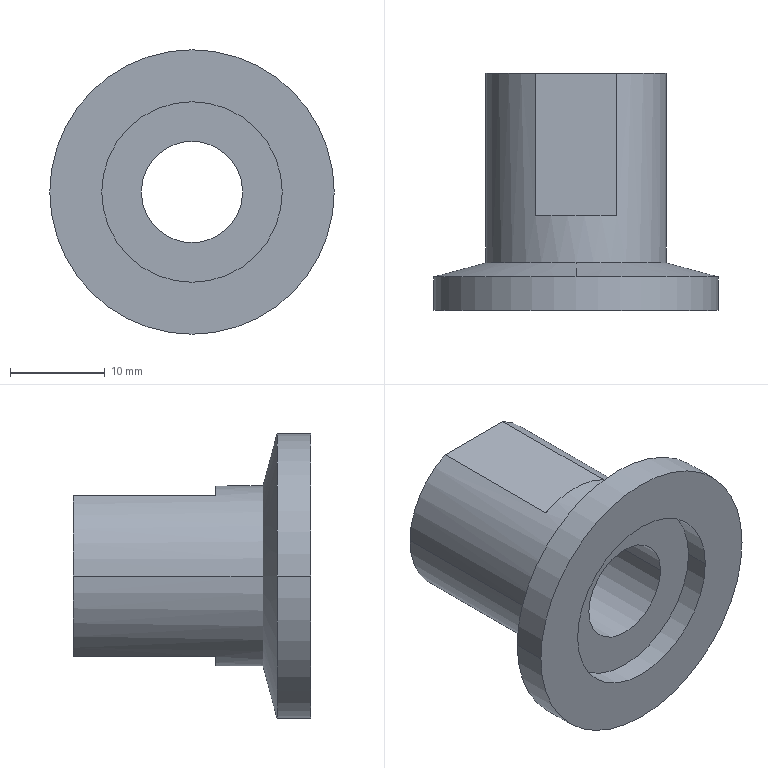Part | SolidWorks | features BaseBody 1 | 1 solid | 20 faces | box 30 x 25 x 30 mm | volume 5740 mm3 | cylinder 8 | plane 8 | cone 4 | commonest cylinder face diameters 19.05 x4 10.7 x2 30 x2
STEP:
#1=CARTESIAN_POINT('',(0.,5.,9.525));
#2=VERTEX_POINT('',#1);
#3=CARTESIAN_POINT('',(9.525,5.,0.));
#4=VERTEX_POINT('',#3);
#5=CARTESIAN_POINT('',(0.,5.,0.));
#6=DIRECTION('',(0.,1.,0.));
#7=DIRECTION('',(-1.,0.,0.));
#8=AXIS2_PLACEMENT_3D('',#5,#6,#7);
#9=CIRCLE('',#8,9.525);
#10=EDGE_CURVE('',#2,#4,#9,.T.);
#11=ORIENTED_EDGE('',*,*,#10,.T.);
#12=CARTESIAN_POINT('',(9.525,25.,0.));
#13=VERTEX_POINT('',#12);
#14=CARTESIAN_POINT('',(9.525,88.82,0.));
#15=DIRECTION('',(0.,1.,0.));
#16=VECTOR('',#15,1000.);
#17=LINE('',#14,#16);
#18=EDGE_CURVE('',#4,#13,#17,.T.);
#19=ORIENTED_EDGE('',*,*,#18,.T.);
#20=CARTESIAN_POINT('',(4.298,25.,8.5));
#21=VERTEX_POINT('',#20);
#22=CARTESIAN_POINT('',(0.,25.,0.));
#23=DIRECTION('',(0.,1.,0.));
#24=DIRECTION('',(-1.,0.,0.));
#25=AXIS2_PLACEMENT_3D('',#22,#23,#24);
#26=CIRCLE('',#25,9.525);
#27=EDGE_CURVE('',#21,#13,#26,.T.);
#28=ORIENTED_EDGE('',*,*,#27,.F.);
#29=CARTESIAN_POINT('',(4.298,10.,8.5));
#30=VERTEX_POINT('',#29);
#31=CARTESIAN_POINT('',(4.298,10.,8.5));
#32=DIRECTION('',(0.,-1.,0.));
#33=VECTOR('',#32,1000.);
#34=LINE('',#31,#33);
#35=EDGE_CURVE('',#21,#30,#34,.T.);
#36=ORIENTED_EDGE('',*,*,#35,.T.);
#37=CARTESIAN_POINT('',(-4.298,10.,8.5));
#38=VERTEX_POINT('',#37);
#39=CARTESIAN_POINT('',(0.,10.,0.));
#40=DIRECTION('',(0.,-1.,0.));
#41=DIRECTION('',(-1.,0.,0.));
#42=AXIS2_PLACEMENT_3D('',#39,#40,#41);
#43=CIRCLE('',#42,9.525);
#44=EDGE_CURVE('',#30,#38,#43,.T.);
#45=ORIENTED_EDGE('',*,*,#44,.T.);
#46=CARTESIAN_POINT('',(-4.298,25.,8.5));
#47=VERTEX_POINT('',#46);
#48=CARTESIAN_POINT('',(-4.298,88.82,8.5));
#49=DIRECTION('',(0.,1.,0.));
#50=VECTOR('',#49,1000.);
#51=LINE('',#48,#50);
#52=EDGE_CURVE('',#38,#47,#51,.T.);
#53=ORIENTED_EDGE('',*,*,#52,.T.);
#54=CARTESIAN_POINT('',(-9.525,25.,0.));
#55=VERTEX_POINT('',#54);
#56=CARTESIAN_POINT('',(0.,25.,0.));
#57=DIRECTION('',(0.,-1.,0.));
#58=DIRECTION('',(-1.,0.,0.));
#59=AXIS2_PLACEMENT_3D('',#56,#57,#58);
#60=CIRCLE('',#59,9.525);
#61=EDGE_CURVE('',#47,#55,#60,.T.);
#62=ORIENTED_EDGE('',*,*,#61,.T.);
#63=CARTESIAN_POINT('',(-9.525,5.,0.));
#64=VERTEX_POINT('',#63);
#65=CARTESIAN_POINT('',(-9.525,88.82,0.));
#66=DIRECTION('',(0.,1.,0.));
#67=VECTOR('',#66,1000.);
#68=LINE('',#65,#67);
#69=EDGE_CURVE('',#64,#55,#68,.T.);
#70=ORIENTED_EDGE('',*,*,#69,.F.);
#71=CARTESIAN_POINT('',(0.,5.,0.));
#72=DIRECTION('',(0.,1.,0.));
#73=DIRECTION('',(-1.,0.,0.));
#74=AXIS2_PLACEMENT_3D('',#71,#72,#73);
#75=CIRCLE('',#74,9.525);
#76=EDGE_CURVE('',#64,#2,#75,.T.);
#77=ORIENTED_EDGE('',*,*,#76,.T.);
#78=EDGE_LOOP('',(#11,#19,#28,#36,#45,#53,#62,#70,#77));
#79=FACE_OUTER_BOUND('',#78,.T.);
#80=CARTESIAN_POINT('',(0.,88.82,0.));
#81=DIRECTION('',(0.,1.,0.));
#82=DIRECTION('',(-1.,0.,0.));
#83=AXIS2_PLACEMENT_3D('',#80,#81,#82);
#84=CYLINDRICAL_SURFACE('',#83,9.525);
#85=ADVANCED_FACE('',(#79),#84,.T.);
#86=ORIENTED_EDGE('',*,*,#10,.F.);
#87=CARTESIAN_POINT('',(0.,3.533,15.));
#88=VERTEX_POINT('',#87);
#89=CARTESIAN_POINT('',(0.,3.533,15.));
#90=DIRECTION('',(0.,-0.2588,0.9659));
#91=VECTOR('',#90,1000.);
#92=LINE('',#89,#91);
#93=EDGE_CURVE('',#2,#88,#92,.T.);
#94=ORIENTED_EDGE('',*,*,#93,.T.);
#95=CARTESIAN_POINT('',(15.,3.533,0.));
#96=VERTEX_POINT('',#95);
#97=CARTESIAN_POINT('',(0.,3.533,0.));
#98=DIRECTION('',(0.,1.,0.));
#99=DIRECTION('',(0.,0.,-1.));
#100=AXIS2_PLACEMENT_3D('',#97,#98,#99);
#101=CIRCLE('',#100,15.);
#102=EDGE_CURVE('',#88,#96,#101,.T.);
#103=ORIENTED_EDGE('',*,*,#102,.T.);
#104=CARTESIAN_POINT('',(0.,3.533,-15.));
#105=VERTEX_POINT('',#104);
#106=CARTESIAN_POINT('',(0.,3.533,0.));
#107=DIRECTION('',(0.,1.,0.));
#108=DIRECTION('',(0.,0.,-1.));
#109=AXIS2_PLACEMENT_3D('',#106,#107,#108);
#110=CIRCLE('',#109,15.);
#111=EDGE_CURVE('',#96,#105,#110,.T.);
#112=ORIENTED_EDGE('',*,*,#111,.T.);
#113=CARTESIAN_POINT('',(0.,5.,-9.525));
#114=VERTEX_POINT('',#113);
#115=CARTESIAN_POINT('',(0.,3.533,-15.));
#116=DIRECTION('',(0.,-0.2588,-0.9659));
#117=VECTOR('',#116,1000.);
#118=LINE('',#115,#117);
#119=EDGE_CURVE('',#114,#105,#118,.T.);
#120=ORIENTED_EDGE('',*,*,#119,.F.);
#121=CARTESIAN_POINT('',(0.,5.,0.));
#122=DIRECTION('',(0.,1.,0.));
#123=DIRECTION('',(-1.,0.,0.));
#124=AXIS2_PLACEMENT_3D('',#121,#122,#123);
#125=CIRCLE('',#124,9.525);
#126=EDGE_CURVE('',#4,#114,#125,.T.);
#127=ORIENTED_EDGE('',*,*,#126,.F.);
#128=EDGE_LOOP('',(#86,#94,#103,#112,#120,#127));
#129=FACE_OUTER_BOUND('',#128,.T.);
#130=CARTESIAN_POINT('',(0.,3.533,0.));
#131=DIRECTION('',(0.,-1.,0.));
#132=DIRECTION('',(0.,0.,-1.));
#133=AXIS2_PLACEMENT_3D('',#130,#131,#132);
#134=CONICAL_SURFACE('',#133,15.,1.309);
#135=ADVANCED_FACE('',(#129),#134,.T.);
#136=CARTESIAN_POINT('',(5.811,14.,0.));
#137=VERTEX_POINT('',#136);
#138=CARTESIAN_POINT('',(-5.811,14.,0.));
#139=VERTEX_POINT('',#138);
#140=CARTESIAN_POINT('',(0.,14.,0.));
#141=DIRECTION('',(0.,1.,0.));
#142=DIRECTION('',(-1.,0.,0.));
#143=AXIS2_PLACEMENT_3D('',#140,#141,#142);
#144=CIRCLE('',#143,5.811);
#145=EDGE_CURVE('',#137,#139,#144,.T.);
#146=ORIENTED_EDGE('',*,*,#145,.F.);
#147=CARTESIAN_POINT('',(6.154,25.,0.));
#148=VERTEX_POINT('',#147);
#149=CARTESIAN_POINT('',(6.154,25.,0.));
#150=DIRECTION('',(0.0312,0.9995,0.));
#151=VECTOR('',#150,1000.);
#152=LINE('',#149,#151);
#153=EDGE_CURVE('',#137,#148,#152,.T.);
#154=ORIENTED_EDGE('',*,*,#153,.T.);
#155=CARTESIAN_POINT('',(-6.154,25.,0.));
#156=VERTEX_POINT('',#155);
#157=CARTESIAN_POINT('',(0.,25.,0.));
#158=DIRECTION('',(0.,-1.,0.));
#159=DIRECTION('',(-1.,0.,0.));
#160=AXIS2_PLACEMENT_3D('',#157,#158,#159);
#161=CIRCLE('',#160,6.154);
#162=EDGE_CURVE('',#156,#148,#161,.T.);
#163=ORIENTED_EDGE('',*,*,#162,.F.);
#164=CARTESIAN_POINT('',(-6.154,25.,0.));
#165=DIRECTION('',(-0.0312,0.9995,0.));
#166=VECTOR('',#165,1000.);
#167=LINE('',#164,#166);
#168=EDGE_CURVE('',#139,#156,#167,.T.);
#169=ORIENTED_EDGE('',*,*,#168,.F.);
#170=EDGE_LOOP('',(#146,#154,#163,#169));
#171=FACE_OUTER_BOUND('',#170,.T.);
#172=CARTESIAN_POINT('',(0.,25.,0.));
#173=DIRECTION('',(0.,1.,0.));
#174=DIRECTION('',(-1.,0.,0.));
#175=AXIS2_PLACEMENT_3D('',#172,#173,#174);
#176=CONICAL_SURFACE('',#175,6.154,0.03121);
#177=ADVANCED_FACE('',(#171),#176,.F.);
#178=CARTESIAN_POINT('',(-15.,0.,0.));
#179=VERTEX_POINT('',#178);
#180=CARTESIAN_POINT('',(15.,0.,0.));
#181=VERTEX_POINT('',#180);
#182=CARTESIAN_POINT('',(0.,0.,0.));
#183=DIRECTION('',(0.,1.,0.));
#184=DIRECTION('',(-1.,0.,0.));
#185=AXIS2_PLACEMENT_3D('',#182,#183,#184);
#186=CIRCLE('',#185,15.);
#187=EDGE_CURVE('',#179,#181,#186,.T.);
#188=ORIENTED_EDGE('',*,*,#187,.T.);
#189=CARTESIAN_POINT('',(15.,88.82,0.));
#190=DIRECTION('',(0.,1.,0.));
#191=VECTOR('',#190,1000.);
#192=LINE('',#189,#191);
#193=EDGE_CURVE('',#181,#96,#192,.T.);
#194=ORIENTED_EDGE('',*,*,#193,.T.);
#195=ORIENTED_EDGE('',*,*,#102,.F.);
#196=CARTESIAN_POINT('',(-15.,3.533,0.));
#197=VERTEX_POINT('',#196);
#198=CARTESIAN_POINT('',(0.,3.533,0.));
#199=DIRECTION('',(0.,1.,0.));
#200=DIRECTION('',(0.,0.,-1.));
#201=AXIS2_PLACEMENT_3D('',#198,#199,#200);
#202=CIRCLE('',#201,15.);
#203=EDGE_CURVE('',#197,#88,#202,.T.);
#204=ORIENTED_EDGE('',*,*,#203,.F.);
#205=CARTESIAN_POINT('',(-15.,88.82,0.));
#206=DIRECTION('',(0.,1.,0.));
#207=VECTOR('',#206,1000.);
#208=LINE('',#205,#207);
#209=EDGE_CURVE('',#179,#197,#208,.T.);
#210=ORIENTED_EDGE('',*,*,#209,.F.);
#211=EDGE_LOOP('',(#188,#194,#195,#204,#210));
#212=FACE_OUTER_BOUND('',#211,.T.);
#213=CARTESIAN_POINT('',(0.,88.82,0.));
#214=DIRECTION('',(0.,1.,0.));
#215=DIRECTION('',(-1.,0.,0.));
#216=AXIS2_PLACEMENT_3D('',#213,#214,#215);
#217=CYLINDRICAL_SURFACE('',#216,15.);
#218=ADVANCED_FACE('',(#212),#217,.T.);
#219=CARTESIAN_POINT('',(5.35,2.5,0.));
#220=VERTEX_POINT('',#219);
#221=CARTESIAN_POINT('',(-5.35,2.5,0.));
#222=VERTEX_POINT('',#221);
#223=CARTESIAN_POINT('',(0.,2.5,0.));
#224=DIRECTION('',(0.,1.,0.));
#225=DIRECTION('',(-1.,0.,0.));
#226=AXIS2_PLACEMENT_3D('',#223,#224,#225);
#227=CIRCLE('',#226,5.35);
#228=EDGE_CURVE('',#220,#222,#227,.T.);
#229=ORIENTED_EDGE('',*,*,#228,.F.);
#230=CARTESIAN_POINT('',(5.35,14.,0.));
#231=VERTEX_POINT('',#230);
#232=CARTESIAN_POINT('',(5.35,25.,0.));
#233=DIRECTION('',(0.,1.,0.));
#234=VECTOR('',#233,1000.);
#235=LINE('',#232,#234);
#236=EDGE_CURVE('',#220,#231,#235,.T.);
#237=ORIENTED_EDGE('',*,*,#236,.T.);
#238=CARTESIAN_POINT('',(-5.35,14.,0.));
#239=VERTEX_POINT('',#238);
#240=CARTESIAN_POINT('',(0.,14.,0.));
#241=DIRECTION('',(0.,1.,0.));
#242=DIRECTION('',(-1.,0.,0.));
#243=AXIS2_PLACEMENT_3D('',#240,#241,#242);
#244=CIRCLE('',#243,5.35);
#245=EDGE_CURVE('',#231,#239,#244,.T.);
#246=ORIENTED_EDGE('',*,*,#245,.T.);
#247=CARTESIAN_POINT('',(-5.35,25.,0.));
#248=DIRECTION('',(0.,1.,0.));
#249=VECTOR('',#248,1000.);
#250=LINE('',#247,#249);
#251=EDGE_CURVE('',#222,#239,#250,.T.);
#252=ORIENTED_EDGE('',*,*,#251,.F.);
#253=EDGE_LOOP('',(#229,#237,#246,#252));
#254=FACE_OUTER_BOUND('',#253,.T.);
#255=CARTESIAN_POINT('',(0.,25.,0.));
#256=DIRECTION('',(0.,1.,0.));
#257=DIRECTION('',(-1.,0.,0.));
#258=AXIS2_PLACEMENT_3D('',#255,#256,#257);
#259=CYLINDRICAL_SURFACE('',#258,5.35);
#260=ADVANCED_FACE('',(#254),#259,.F.);
#261=CARTESIAN_POINT('',(9.525,0.,0.));
#262=VERTEX_POINT('',#261);
#263=CARTESIAN_POINT('',(-9.525,0.,0.));
#264=VERTEX_POINT('',#263);
#265=CARTESIAN_POINT('',(0.,0.,0.));
#266=DIRECTION('',(0.,1.,0.));
#267=DIRECTION('',(-1.,0.,0.));
#268=AXIS2_PLACEMENT_3D('',#265,#266,#267);
#269=CIRCLE('',#268,9.525);
#270=EDGE_CURVE('',#262,#264,#269,.T.);
#271=ORIENTED_EDGE('',*,*,#270,.F.);
#272=CARTESIAN_POINT('',(9.525,2.5,0.));
#273=VERTEX_POINT('',#272);
#274=CARTESIAN_POINT('',(9.525,88.82,0.));
#275=DIRECTION('',(0.,1.,0.));
#276=VECTOR('',#275,1000.);
#277=LINE('',#274,#276);
#278=EDGE_CURVE('',#262,#273,#277,.T.);
#279=ORIENTED_EDGE('',*,*,#278,.T.);
#280=CARTESIAN_POINT('',(-9.525,2.5,0.));
#281=VERTEX_POINT('',#280);
#282=CARTESIAN_POINT('',(0.,2.5,0.));
#283=DIRECTION('',(0.,-1.,0.));
#284=DIRECTION('',(-1.,0.,0.));
#285=AXIS2_PLACEMENT_3D('',#282,#283,#284);
#286=CIRCLE('',#285,9.525);
#287=EDGE_CURVE('',#281,#273,#286,.T.);
#288=ORIENTED_EDGE('',*,*,#287,.F.);
#289=CARTESIAN_POINT('',(-9.525,88.82,0.));
#290=DIRECTION('',(0.,1.,0.));
#291=VECTOR('',#290,1000.);
#292=LINE('',#289,#291);
#293=EDGE_CURVE('',#264,#281,#292,.T.);
#294=ORIENTED_EDGE('',*,*,#293,.F.);
#295=EDGE_LOOP('',(#271,#279,#288,#294));
#296=FACE_OUTER_BOUND('',#295,.T.);
#297=CARTESIAN_POINT('',(0.,88.82,0.));
#298=DIRECTION('',(0.,1.,0.));
#299=DIRECTION('',(-1.,0.,0.));
#300=AXIS2_PLACEMENT_3D('',#297,#298,#299);
#301=CYLINDRICAL_SURFACE('',#300,9.525);
#302=ADVANCED_FACE('',(#296),#301,.F.);
#303=ORIENTED_EDGE('',*,*,#18,.F.);
#304=ORIENTED_EDGE('',*,*,#126,.T.);
#305=CARTESIAN_POINT('',(0.,5.,0.));
#306=DIRECTION('',(0.,1.,0.));
#307=DIRECTION('',(-1.,0.,0.));
#308=AXIS2_PLACEMENT_3D('',#305,#306,#307);
#309=CIRCLE('',#308,9.525);
#310=EDGE_CURVE('',#114,#64,#309,.T.);
#311=ORIENTED_EDGE('',*,*,#310,.T.);
#312=ORIENTED_EDGE('',*,*,#69,.T.);
#313=CARTESIAN_POINT('',(-4.298,25.,-8.5));
#314=VERTEX_POINT('',#313);
#315=CARTESIAN_POINT('',(0.,25.,0.));
#316=DIRECTION('',(0.,-1.,0.));
#317=DIRECTION('',(-1.,0.,0.));
#318=AXIS2_PLACEMENT_3D('',#315,#316,#317);
#319=CIRCLE('',#318,9.525);
#320=EDGE_CURVE('',#55,#314,#319,.T.);
#321=ORIENTED_EDGE('',*,*,#320,.T.);
#322=CARTESIAN_POINT('',(-4.298,10.,-8.5));
#323=VERTEX_POINT('',#322);
#324=CARTESIAN_POINT('',(-4.298,88.82,-8.5));
#325=DIRECTION('',(0.,-1.,0.));
#326=VECTOR('',#325,1000.);
#327=LINE('',#324,#326);
#328=EDGE_CURVE('',#314,#323,#327,.T.);
#329=ORIENTED_EDGE('',*,*,#328,.T.);
#330=CARTESIAN_POINT('',(4.298,10.,-8.5));
#331=VERTEX_POINT('',#330);
#332=CARTESIAN_POINT('',(0.,10.,0.));
#333=DIRECTION('',(0.,-1.,0.));
#334=DIRECTION('',(-1.,0.,0.));
#335=AXIS2_PLACEMENT_3D('',#332,#333,#334);
#336=CIRCLE('',#335,9.525);
#337=EDGE_CURVE('',#323,#331,#336,.T.);
#338=ORIENTED_EDGE('',*,*,#337,.T.);
#339=CARTESIAN_POINT('',(4.298,25.,-8.5));
#340=VERTEX_POINT('',#339);
#341=CARTESIAN_POINT('',(4.298,10.,-8.5));
#342=DIRECTION('',(0.,1.,0.));
#343=VECTOR('',#342,1000.);
#344=LINE('',#341,#343);
#345=EDGE_CURVE('',#331,#340,#344,.T.);
#346=ORIENTED_EDGE('',*,*,#345,.T.);
#347=CARTESIAN_POINT('',(0.,25.,0.));
#348=DIRECTION('',(0.,1.,0.));
#349=DIRECTION('',(-1.,0.,0.));
#350=AXIS2_PLACEMENT_3D('',#347,#348,#349);
#351=CIRCLE('',#350,9.525);
#352=EDGE_CURVE('',#13,#340,#351,.T.);
#353=ORIENTED_EDGE('',*,*,#352,.F.);
#354=EDGE_LOOP('',(#303,#304,#311,#312,#321,#329,#338,#346,#353));
#355=FACE_OUTER_BOUND('',#354,.T.);
#356=CARTESIAN_POINT('',(0.,88.82,0.));
#357=DIRECTION('',(0.,1.,0.));
#358=DIRECTION('',(-1.,0.,0.));
#359=AXIS2_PLACEMENT_3D('',#356,#357,#358);
#360=CYLINDRICAL_SURFACE('',#359,9.525);
#361=ADVANCED_FACE('',(#355),#360,.T.);
#362=CARTESIAN_POINT('',(0.,10.,-8.5));
#363=DIRECTION('',(1.,0.,0.));
#364=VECTOR('',#363,1000.);
#365=LINE('',#362,#364);
#366=EDGE_CURVE('',#323,#331,#365,.T.);
#367=ORIENTED_EDGE('',*,*,#366,.T.);
#368=ORIENTED_EDGE('',*,*,#337,.F.);
#369=EDGE_LOOP('',(#367,#368));
#370=FACE_OUTER_BOUND('',#369,.T.);
#371=CARTESIAN_POINT('',(0.,10.,0.));
#372=DIRECTION('',(0.,1.,0.));
#373=DIRECTION('',(-1.,0.,0.));
#374=AXIS2_PLACEMENT_3D('',#371,#372,#373);
#375=PLANE('',#374);
#376=ADVANCED_FACE('',(#370),#375,.T.);
#377=ORIENTED_EDGE('',*,*,#366,.F.);
#378=ORIENTED_EDGE('',*,*,#328,.F.);
#379=CARTESIAN_POINT('',(-19.454,25.,-8.5));
#380=DIRECTION('',(-1.,0.,0.));
#381=VECTOR('',#380,1000.);
#382=LINE('',#379,#381);
#383=EDGE_CURVE('',#340,#314,#382,.T.);
#384=ORIENTED_EDGE('',*,*,#383,.F.);
#385=ORIENTED_EDGE('',*,*,#345,.F.);
#386=EDGE_LOOP('',(#377,#378,#384,#385));
#387=FACE_OUTER_BOUND('',#386,.T.);
#388=CARTESIAN_POINT('',(-19.454,10.,-8.5));
#389=DIRECTION('',(0.,0.,1.));
#390=DIRECTION('',(1.,0.,0.));
#391=AXIS2_PLACEMENT_3D('',#388,#389,#390);
#392=PLANE('',#391);
#393=ADVANCED_FACE('',(#387),#392,.F.);
#394=ORIENTED_EDGE('',*,*,#162,.T.);
#395=CARTESIAN_POINT('',(0.,25.,0.));
#396=DIRECTION('',(0.,-1.,0.));
#397=DIRECTION('',(-1.,0.,0.));
#398=AXIS2_PLACEMENT_3D('',#395,#396,#397);
#399=CIRCLE('',#398,6.154);
#400=EDGE_CURVE('',#148,#156,#399,.T.);
#401=ORIENTED_EDGE('',*,*,#400,.T.);
#402=EDGE_LOOP('',(#394,#401));
#403=FACE_BOUND('',#402,.T.);
#404=ORIENTED_EDGE('',*,*,#383,.T.);
#405=ORIENTED_EDGE('',*,*,#320,.F.);
#406=ORIENTED_EDGE('',*,*,#61,.F.);
#407=CARTESIAN_POINT('',(-9.525,25.,8.5));
#408=DIRECTION('',(1.,0.,0.));
#409=VECTOR('',#408,1000.);
#410=LINE('',#407,#409);
#411=EDGE_CURVE('',#47,#21,#410,.T.);
#412=ORIENTED_EDGE('',*,*,#411,.T.);
#413=ORIENTED_EDGE('',*,*,#27,.T.);
#414=ORIENTED_EDGE('',*,*,#352,.T.);
#415=EDGE_LOOP('',(#404,#405,#406,#412,#413,#414));
#416=FACE_OUTER_BOUND('',#415,.T.);
#417=CARTESIAN_POINT('',(-9.525,25.,0.));
#418=DIRECTION('',(0.,1.,0.));
#419=DIRECTION('',(-1.,0.,0.));
#420=AXIS2_PLACEMENT_3D('',#417,#418,#419);
#421=PLANE('',#420);
#422=ADVANCED_FACE('',(#403,#416),#421,.T.);
#423=CARTESIAN_POINT('',(-30.646,10.,8.5));
#424=DIRECTION('',(-1.,0.,0.));
#425=VECTOR('',#424,1000.);
#426=LINE('',#423,#425);
#427=EDGE_CURVE('',#30,#38,#426,.T.);
#428=ORIENTED_EDGE('',*,*,#427,.F.);
#429=ORIENTED_EDGE('',*,*,#35,.F.);
#430=ORIENTED_EDGE('',*,*,#411,.F.);
#431=ORIENTED_EDGE('',*,*,#52,.F.);
#432=EDGE_LOOP('',(#428,#429,#430,#431));
#433=FACE_OUTER_BOUND('',#432,.T.);
#434=CARTESIAN_POINT('',(-30.646,10.,8.5));
#435=DIRECTION('',(0.,0.,-1.));
#436=DIRECTION('',(-1.,0.,0.));
#437=AXIS2_PLACEMENT_3D('',#434,#435,#436);
#438=PLANE('',#437);
#439=ADVANCED_FACE('',(#433),#438,.F.);
#440=ORIENTED_EDGE('',*,*,#44,.F.);
#441=ORIENTED_EDGE('',*,*,#427,.T.);
#442=EDGE_LOOP('',(#440,#441));
#443=FACE_OUTER_BOUND('',#442,.T.);
#444=CARTESIAN_POINT('',(0.,10.,0.));
#445=DIRECTION('',(0.,1.,0.));
#446=DIRECTION('',(-1.,0.,0.));
#447=AXIS2_PLACEMENT_3D('',#444,#445,#446);
#448=PLANE('',#447);
#449=ADVANCED_FACE('',(#443),#448,.T.);
#450=ORIENTED_EDGE('',*,*,#93,.F.);
#451=ORIENTED_EDGE('',*,*,#76,.F.);
#452=ORIENTED_EDGE('',*,*,#310,.F.);
#453=ORIENTED_EDGE('',*,*,#119,.T.);
#454=CARTESIAN_POINT('',(0.,3.533,0.));
#455=DIRECTION('',(0.,1.,0.));
#456=DIRECTION('',(0.,0.,-1.));
#457=AXIS2_PLACEMENT_3D('',#454,#455,#456);
#458=CIRCLE('',#457,15.);
#459=EDGE_CURVE('',#105,#197,#458,.T.);
#460=ORIENTED_EDGE('',*,*,#459,.T.);
#461=ORIENTED_EDGE('',*,*,#203,.T.);
#462=EDGE_LOOP('',(#450,#451,#452,#453,#460,#461));
#463=FACE_OUTER_BOUND('',#462,.T.);
#464=CARTESIAN_POINT('',(0.,3.533,0.));
#465=DIRECTION('',(0.,-1.,0.));
#466=DIRECTION('',(0.,0.,-1.));
#467=AXIS2_PLACEMENT_3D('',#464,#465,#466);
#468=CONICAL_SURFACE('',#467,15.,1.309);
#469=ADVANCED_FACE('',(#463),#468,.T.);
#470=ORIENTED_EDGE('',*,*,#153,.F.);
#471=CARTESIAN_POINT('',(0.,14.,0.));
#472=DIRECTION('',(0.,1.,0.));
#473=DIRECTION('',(-1.,0.,0.));
#474=AXIS2_PLACEMENT_3D('',#471,#472,#473);
#475=CIRCLE('',#474,5.811);
#476=EDGE_CURVE('',#139,#137,#475,.T.);
#477=ORIENTED_EDGE('',*,*,#476,.F.);
#478=ORIENTED_EDGE('',*,*,#168,.T.);
#479=ORIENTED_EDGE('',*,*,#400,.F.);
#480=EDGE_LOOP('',(#470,#477,#478,#479));
#481=FACE_OUTER_BOUND('',#480,.T.);
#482=CARTESIAN_POINT('',(0.,25.,0.));
#483=DIRECTION('',(0.,1.,0.));
#484=DIRECTION('',(-1.,0.,0.));
#485=AXIS2_PLACEMENT_3D('',#482,#483,#484);
#486=CONICAL_SURFACE('',#485,6.154,0.03121);
#487=ADVANCED_FACE('',(#481),#486,.F.);
#488=ORIENTED_EDGE('',*,*,#193,.F.);
#489=CARTESIAN_POINT('',(0.,0.,0.));
#490=DIRECTION('',(0.,1.,0.));
#491=DIRECTION('',(-1.,0.,0.));
#492=AXIS2_PLACEMENT_3D('',#489,#490,#491);
#493=CIRCLE('',#492,15.);
#494=EDGE_CURVE('',#181,#179,#493,.T.);
#495=ORIENTED_EDGE('',*,*,#494,.T.);
#496=ORIENTED_EDGE('',*,*,#209,.T.);
#497=ORIENTED_EDGE('',*,*,#459,.F.);
#498=ORIENTED_EDGE('',*,*,#111,.F.);
#499=EDGE_LOOP('',(#488,#495,#496,#497,#498));
#500=FACE_OUTER_BOUND('',#499,.T.);
#501=CARTESIAN_POINT('',(0.,88.82,0.));
#502=DIRECTION('',(0.,1.,0.));
#503=DIRECTION('',(-1.,0.,0.));
#504=AXIS2_PLACEMENT_3D('',#501,#502,#503);
#505=CYLINDRICAL_SURFACE('',#504,15.);
#506=ADVANCED_FACE('',(#500),#505,.T.);
#507=ORIENTED_EDGE('',*,*,#476,.T.);
#508=ORIENTED_EDGE('',*,*,#145,.T.);
#509=EDGE_LOOP('',(#507,#508));
#510=FACE_OUTER_BOUND('',#509,.T.);
#511=CARTESIAN_POINT('',(0.,14.,0.));
#512=DIRECTION('',(0.,1.,0.));
#513=DIRECTION('',(-1.,0.,0.));
#514=AXIS2_PLACEMENT_3D('',#511,#512,#513);
#515=CIRCLE('',#514,5.35);
#516=EDGE_CURVE('',#239,#231,#515,.T.);
#517=ORIENTED_EDGE('',*,*,#516,.F.);
#518=ORIENTED_EDGE('',*,*,#245,.F.);
#519=EDGE_LOOP('',(#517,#518));
#520=FACE_BOUND('',#519,.T.);
#521=CARTESIAN_POINT('',(5.35,14.,0.));
#522=DIRECTION('',(0.,-1.,0.));
#523=DIRECTION('',(1.,0.,0.));
#524=AXIS2_PLACEMENT_3D('',#521,#522,#523);
#525=PLANE('',#524);
#526=ADVANCED_FACE('',(#510,#520),#525,.F.);
#527=ORIENTED_EDGE('',*,*,#187,.F.);
#528=ORIENTED_EDGE('',*,*,#494,.F.);
#529=EDGE_LOOP('',(#527,#528));
#530=FACE_OUTER_BOUND('',#529,.T.);
#531=CARTESIAN_POINT('',(0.,0.,0.));
#532=DIRECTION('',(0.,1.,0.));
#533=DIRECTION('',(-1.,0.,0.));
#534=AXIS2_PLACEMENT_3D('',#531,#532,#533);
#535=CIRCLE('',#534,9.525);
#536=EDGE_CURVE('',#264,#262,#535,.T.);
#537=ORIENTED_EDGE('',*,*,#536,.T.);
#538=ORIENTED_EDGE('',*,*,#270,.T.);
#539=EDGE_LOOP('',(#537,#538));
#540=FACE_BOUND('',#539,.T.);
#541=CARTESIAN_POINT('',(-15.,0.,0.));
#542=DIRECTION('',(0.,-1.,0.));
#543=DIRECTION('',(1.,0.,0.));
#544=AXIS2_PLACEMENT_3D('',#541,#542,#543);
#545=PLANE('',#544);
#546=ADVANCED_FACE('',(#530,#540),#545,.T.);
#547=ORIENTED_EDGE('',*,*,#236,.F.);
#548=CARTESIAN_POINT('',(0.,2.5,0.));
#549=DIRECTION('',(0.,1.,0.));
#550=DIRECTION('',(-1.,0.,0.));
#551=AXIS2_PLACEMENT_3D('',#548,#549,#550);
#552=CIRCLE('',#551,5.35);
#553=EDGE_CURVE('',#222,#220,#552,.T.);
#554=ORIENTED_EDGE('',*,*,#553,.F.);
#555=ORIENTED_EDGE('',*,*,#251,.T.);
#556=ORIENTED_EDGE('',*,*,#516,.T.);
#557=EDGE_LOOP('',(#547,#554,#555,#556));
#558=FACE_OUTER_BOUND('',#557,.T.);
#559=CARTESIAN_POINT('',(0.,25.,0.));
#560=DIRECTION('',(0.,1.,0.));
#561=DIRECTION('',(-1.,0.,0.));
#562=AXIS2_PLACEMENT_3D('',#559,#560,#561);
#563=CYLINDRICAL_SURFACE('',#562,5.35);
#564=ADVANCED_FACE('',(#558),#563,.F.);
#565=ORIENTED_EDGE('',*,*,#278,.F.);
#566=ORIENTED_EDGE('',*,*,#536,.F.);
#567=ORIENTED_EDGE('',*,*,#293,.T.);
#568=CARTESIAN_POINT('',(0.,2.5,0.));
#569=DIRECTION('',(0.,-1.,0.));
#570=DIRECTION('',(-1.,0.,0.));
#571=AXIS2_PLACEMENT_3D('',#568,#569,#570);
#572=CIRCLE('',#571,9.525);
#573=EDGE_CURVE('',#273,#281,#572,.T.);
#574=ORIENTED_EDGE('',*,*,#573,.F.);
#575=EDGE_LOOP('',(#565,#566,#567,#574));
#576=FACE_OUTER_BOUND('',#575,.T.);
#577=CARTESIAN_POINT('',(0.,88.82,0.));
#578=DIRECTION('',(0.,1.,0.));
#579=DIRECTION('',(-1.,0.,0.));
#580=AXIS2_PLACEMENT_3D('',#577,#578,#579);
#581=CYLINDRICAL_SURFACE('',#580,9.525);
#582=ADVANCED_FACE('',(#576),#581,.F.);
#583=ORIENTED_EDGE('',*,*,#287,.T.);
#584=ORIENTED_EDGE('',*,*,#573,.T.);
#585=EDGE_LOOP('',(#583,#584));
#586=FACE_OUTER_BOUND('',#585,.T.);
#587=ORIENTED_EDGE('',*,*,#553,.T.);
#588=ORIENTED_EDGE('',*,*,#228,.T.);
#589=EDGE_LOOP('',(#587,#588));
#590=FACE_BOUND('',#589,.T.);
#591=CARTESIAN_POINT('',(-9.525,2.5,0.));
#592=DIRECTION('',(0.,-1.,0.));
#593=DIRECTION('',(1.,0.,0.));
#594=AXIS2_PLACEMENT_3D('',#591,#592,#593);
#595=PLANE('',#594);
#596=ADVANCED_FACE('',(#586,#590),#595,.T.);
#597=CLOSED_SHELL('',(#85,#135,#177,#218,#260,#302,#361,#376,#393,#422,#439,#449,#469,#487,#506,#526,#546,#564,#582,#596));
#598=MANIFOLD_SOLID_BREP('',#597);
#599=CARTESIAN_POINT('',(0.,0.,0.));
#600=DIRECTION('',(0.,0.,1.));
#601=DIRECTION('',(1.,0.,0.));
#602=AXIS2_PLACEMENT_3D('',#599,#600,#601);
#603=(LENGTH_UNIT()NAMED_UNIT(*)SI_UNIT(.MILLI.,.METRE.));
#604=UNCERTAINTY_MEASURE_WITH_UNIT(LENGTH_MEASURE(0.00001),#603,'','');
#605=(NAMED_UNIT(*)PLANE_ANGLE_UNIT()SI_UNIT($,.RADIAN.));
#606=(NAMED_UNIT(*)SI_UNIT($,.STERADIAN.)SOLID_ANGLE_UNIT());
#607=(GEOMETRIC_REPRESENTATION_CONTEXT(3)GLOBAL_UNCERTAINTY_ASSIGNED_CONTEXT((#604))GLOBAL_UNIT_ASSIGNED_CONTEXT((#603,#605,#606))REPRESENTATION_CONTEXT('',''));
#608=ADVANCED_BREP_SHAPE_REPRESENTATION('',(#598,#602),#607);